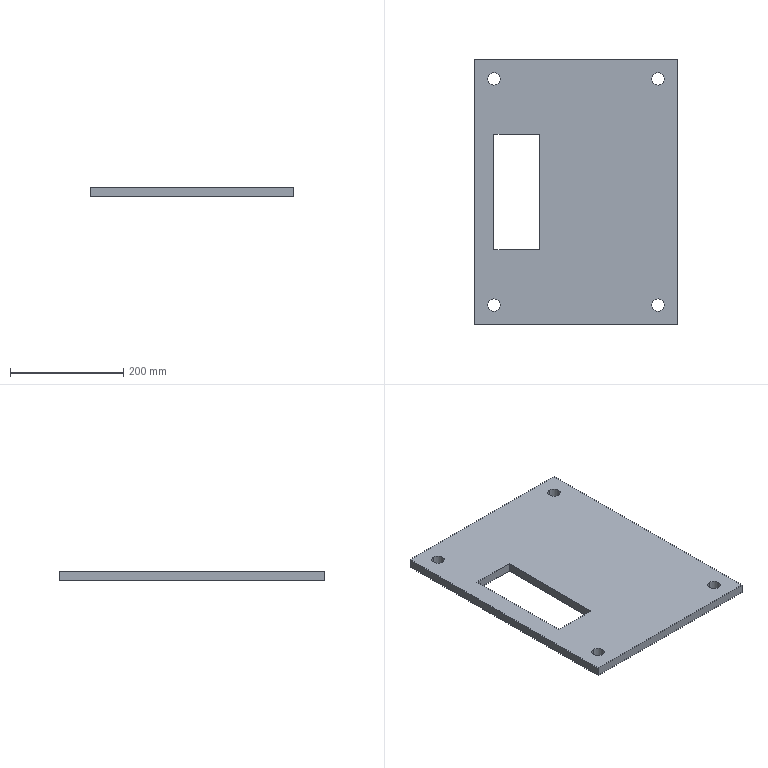Part | STEP file | 05-Base plate | 1 solid | 18 faces | box 360 x 470 x 16 mm | volume 2420472 mm3 | plane 10 | cylinder 8 | commonest cylinder face diameters 22 x8
STEP:
#1=CARTESIAN_POINT('',(0.,0.,0.));
#2=DIRECTION('',(0.,0.,1.));
#3=DIRECTION('',(1.,0.,0.));
#4=AXIS2_PLACEMENT_3D('',#1,#2,#3);
#5=CARTESIAN_POINT('',(35.,-446.,0.));
#6=VERTEX_POINT('',#5);
#7=CARTESIAN_POINT('',(35.,-446.,16.));
#8=VERTEX_POINT('',#7);
#9=CARTESIAN_POINT('',(35.,-446.,-44.));
#10=DIRECTION('',(0.,0.,1.));
#11=VECTOR('',#10,1.);
#12=LINE('',#9,#11);
#13=CARTESIAN_POINT('',(35.,-435.,-44.));
#14=DIRECTION('',(0.,0.,1.));
#15=DIRECTION('',(0.,-1.,0.));
#16=AXIS2_PLACEMENT_3D('',#13,#14,#15);
#17=CYLINDRICAL_SURFACE('',#16,11.);
#18=CARTESIAN_POINT('',(6.283,0.));
#19=DIRECTION('',(0.,1.));
#20=VECTOR('',#19,1.);
#21=LINE('',#18,#20);
#22=(GEOMETRIC_REPRESENTATION_CONTEXT(2)PARAMETRIC_REPRESENTATION_CONTEXT()REPRESENTATION_CONTEXT('',''));
#23=DEFINITIONAL_REPRESENTATION('',(#21),#22);
#24=PCURVE('',#17,#23);
#25=CARTESIAN_POINT('',(35.,-435.,-44.));
#26=DIRECTION('',(0.,0.,1.));
#27=DIRECTION('',(0.,-1.,0.));
#28=AXIS2_PLACEMENT_3D('',#25,#26,#27);
#29=CYLINDRICAL_SURFACE('',#28,11.);
#30=CARTESIAN_POINT('',(0.,0.));
#31=DIRECTION('',(0.,1.));
#32=VECTOR('',#31,1.);
#33=LINE('',#30,#32);
#34=(GEOMETRIC_REPRESENTATION_CONTEXT(2)PARAMETRIC_REPRESENTATION_CONTEXT()REPRESENTATION_CONTEXT('',''));
#35=DEFINITIONAL_REPRESENTATION('',(#33),#34);
#36=PCURVE('',#29,#35);
#37=SURFACE_CURVE('',#12,(#24,#36),.PCURVE_S1.);
#38=EDGE_CURVE('',#6,#8,#37,.T.);
#39=ORIENTED_EDGE('',*,*,#38,.T.);
#40=CARTESIAN_POINT('',(35.,-424.,16.));
#41=VERTEX_POINT('',#40);
#42=CARTESIAN_POINT('',(35.,-435.,16.));
#43=DIRECTION('',(0.,0.,1.));
#44=DIRECTION('',(0.,-1.,0.));
#45=AXIS2_PLACEMENT_3D('',#42,#43,#44);
#46=CIRCLE('',#45,11.);
#47=CARTESIAN_POINT('',(0.,60.));
#48=DIRECTION('',(1.,0.));
#49=VECTOR('',#48,1.);
#50=LINE('',#47,#49);
#51=(GEOMETRIC_REPRESENTATION_CONTEXT(2)PARAMETRIC_REPRESENTATION_CONTEXT()REPRESENTATION_CONTEXT('',''));
#52=DEFINITIONAL_REPRESENTATION('',(#50),#51);
#53=PCURVE('',#17,#52);
#54=CARTESIAN_POINT('',(0.,0.,16.));
#55=DIRECTION('',(0.,0.,1.));
#56=DIRECTION('',(1.,0.,0.));
#57=AXIS2_PLACEMENT_3D('',#54,#55,#56);
#58=PLANE('',#57);
#59=CARTESIAN_POINT('',(35.,-435.));
#60=DIRECTION('',(0.,-1.));
#61=AXIS2_PLACEMENT_2D('',#59,#60);
#62=CIRCLE('',#61,11.);
#63=(GEOMETRIC_REPRESENTATION_CONTEXT(2)PARAMETRIC_REPRESENTATION_CONTEXT()REPRESENTATION_CONTEXT('',''));
#64=DEFINITIONAL_REPRESENTATION('',(#62),#63);
#65=PCURVE('',#58,#64);
#66=SURFACE_CURVE('',#46,(#53,#65),.PCURVE_S1.);
#67=EDGE_CURVE('',#41,#8,#66,.T.);
#68=ORIENTED_EDGE('',*,*,#67,.F.);
#69=CARTESIAN_POINT('',(35.,-424.,0.));
#70=VERTEX_POINT('',#69);
#71=CARTESIAN_POINT('',(35.,-424.,-44.));
#72=DIRECTION('',(0.,0.,1.));
#73=VECTOR('',#72,1.);
#74=LINE('',#71,#73);
#75=CARTESIAN_POINT('',(3.142,0.));
#76=DIRECTION('',(0.,1.));
#77=VECTOR('',#76,1.);
#78=LINE('',#75,#77);
#79=(GEOMETRIC_REPRESENTATION_CONTEXT(2)PARAMETRIC_REPRESENTATION_CONTEXT()REPRESENTATION_CONTEXT('',''));
#80=DEFINITIONAL_REPRESENTATION('',(#78),#79);
#81=PCURVE('',#17,#80);
#82=CARTESIAN_POINT('',(3.142,0.));
#83=DIRECTION('',(0.,1.));
#84=VECTOR('',#83,1.);
#85=LINE('',#82,#84);
#86=(GEOMETRIC_REPRESENTATION_CONTEXT(2)PARAMETRIC_REPRESENTATION_CONTEXT()REPRESENTATION_CONTEXT('',''));
#87=DEFINITIONAL_REPRESENTATION('',(#85),#86);
#88=PCURVE('',#29,#87);
#89=SURFACE_CURVE('',#74,(#81,#88),.PCURVE_S1.);
#90=EDGE_CURVE('',#70,#41,#89,.T.);
#91=ORIENTED_EDGE('',*,*,#90,.F.);
#92=CARTESIAN_POINT('',(35.,-435.,0.));
#93=DIRECTION('',(0.,0.,1.));
#94=DIRECTION('',(0.,-1.,0.));
#95=AXIS2_PLACEMENT_3D('',#92,#93,#94);
#96=CIRCLE('',#95,11.);
#97=CARTESIAN_POINT('',(0.,44.));
#98=DIRECTION('',(1.,0.));
#99=VECTOR('',#98,1.);
#100=LINE('',#97,#99);
#101=(GEOMETRIC_REPRESENTATION_CONTEXT(2)PARAMETRIC_REPRESENTATION_CONTEXT()REPRESENTATION_CONTEXT('',''));
#102=DEFINITIONAL_REPRESENTATION('',(#100),#101);
#103=PCURVE('',#17,#102);
#104=CARTESIAN_POINT('',(0.,0.,0.));
#105=DIRECTION('',(0.,0.,1.));
#106=DIRECTION('',(1.,0.,0.));
#107=AXIS2_PLACEMENT_3D('',#104,#105,#106);
#108=PLANE('',#107);
#109=CARTESIAN_POINT('',(35.,-435.));
#110=DIRECTION('',(0.,-1.));
#111=AXIS2_PLACEMENT_2D('',#109,#110);
#112=CIRCLE('',#111,11.);
#113=(GEOMETRIC_REPRESENTATION_CONTEXT(2)PARAMETRIC_REPRESENTATION_CONTEXT()REPRESENTATION_CONTEXT('',''));
#114=DEFINITIONAL_REPRESENTATION('',(#112),#113);
#115=PCURVE('',#108,#114);
#116=SURFACE_CURVE('',#96,(#103,#115),.PCURVE_S1.);
#117=EDGE_CURVE('',#70,#6,#116,.T.);
#118=ORIENTED_EDGE('',*,*,#117,.T.);
#119=EDGE_LOOP('',(#39,#68,#91,#118));
#120=FACE_BOUND('',#119,.F.);
#121=ADVANCED_FACE('',(#120),#17,.F.);
#122=CARTESIAN_POINT('',(325.,-446.,0.));
#123=VERTEX_POINT('',#122);
#124=CARTESIAN_POINT('',(325.,-446.,16.));
#125=VERTEX_POINT('',#124);
#126=CARTESIAN_POINT('',(325.,-446.,-44.));
#127=DIRECTION('',(0.,0.,1.));
#128=VECTOR('',#127,1.);
#129=LINE('',#126,#128);
#130=CARTESIAN_POINT('',(325.,-435.,-44.));
#131=DIRECTION('',(0.,0.,1.));
#132=DIRECTION('',(0.,-1.,0.));
#133=AXIS2_PLACEMENT_3D('',#130,#131,#132);
#134=CYLINDRICAL_SURFACE('',#133,11.);
#135=CARTESIAN_POINT('',(6.283,0.));
#136=DIRECTION('',(0.,1.));
#137=VECTOR('',#136,1.);
#138=LINE('',#135,#137);
#139=(GEOMETRIC_REPRESENTATION_CONTEXT(2)PARAMETRIC_REPRESENTATION_CONTEXT()REPRESENTATION_CONTEXT('',''));
#140=DEFINITIONAL_REPRESENTATION('',(#138),#139);
#141=PCURVE('',#134,#140);
#142=CARTESIAN_POINT('',(325.,-435.,-44.));
#143=DIRECTION('',(0.,0.,1.));
#144=DIRECTION('',(0.,-1.,0.));
#145=AXIS2_PLACEMENT_3D('',#142,#143,#144);
#146=CYLINDRICAL_SURFACE('',#145,11.);
#147=CARTESIAN_POINT('',(0.,0.));
#148=DIRECTION('',(0.,1.));
#149=VECTOR('',#148,1.);
#150=LINE('',#147,#149);
#151=(GEOMETRIC_REPRESENTATION_CONTEXT(2)PARAMETRIC_REPRESENTATION_CONTEXT()REPRESENTATION_CONTEXT('',''));
#152=DEFINITIONAL_REPRESENTATION('',(#150),#151);
#153=PCURVE('',#146,#152);
#154=SURFACE_CURVE('',#129,(#141,#153),.PCURVE_S1.);
#155=EDGE_CURVE('',#123,#125,#154,.T.);
#156=ORIENTED_EDGE('',*,*,#155,.T.);
#157=CARTESIAN_POINT('',(325.,-424.,16.));
#158=VERTEX_POINT('',#157);
#159=CARTESIAN_POINT('',(325.,-435.,16.));
#160=DIRECTION('',(0.,0.,1.));
#161=DIRECTION('',(0.,-1.,0.));
#162=AXIS2_PLACEMENT_3D('',#159,#160,#161);
#163=CIRCLE('',#162,11.);
#164=CARTESIAN_POINT('',(0.,60.));
#165=DIRECTION('',(1.,0.));
#166=VECTOR('',#165,1.);
#167=LINE('',#164,#166);
#168=(GEOMETRIC_REPRESENTATION_CONTEXT(2)PARAMETRIC_REPRESENTATION_CONTEXT()REPRESENTATION_CONTEXT('',''));
#169=DEFINITIONAL_REPRESENTATION('',(#167),#168);
#170=PCURVE('',#134,#169);
#171=CARTESIAN_POINT('',(325.,-435.));
#172=DIRECTION('',(0.,-1.));
#173=AXIS2_PLACEMENT_2D('',#171,#172);
#174=CIRCLE('',#173,11.);
#175=(GEOMETRIC_REPRESENTATION_CONTEXT(2)PARAMETRIC_REPRESENTATION_CONTEXT()REPRESENTATION_CONTEXT('',''));
#176=DEFINITIONAL_REPRESENTATION('',(#174),#175);
#177=PCURVE('',#58,#176);
#178=SURFACE_CURVE('',#163,(#170,#177),.PCURVE_S1.);
#179=EDGE_CURVE('',#158,#125,#178,.T.);
#180=ORIENTED_EDGE('',*,*,#179,.F.);
#181=CARTESIAN_POINT('',(325.,-424.,0.));
#182=VERTEX_POINT('',#181);
#183=CARTESIAN_POINT('',(325.,-424.,-44.));
#184=DIRECTION('',(0.,0.,1.));
#185=VECTOR('',#184,1.);
#186=LINE('',#183,#185);
#187=CARTESIAN_POINT('',(3.142,0.));
#188=DIRECTION('',(0.,1.));
#189=VECTOR('',#188,1.);
#190=LINE('',#187,#189);
#191=(GEOMETRIC_REPRESENTATION_CONTEXT(2)PARAMETRIC_REPRESENTATION_CONTEXT()REPRESENTATION_CONTEXT('',''));
#192=DEFINITIONAL_REPRESENTATION('',(#190),#191);
#193=PCURVE('',#134,#192);
#194=CARTESIAN_POINT('',(3.142,0.));
#195=DIRECTION('',(0.,1.));
#196=VECTOR('',#195,1.);
#197=LINE('',#194,#196);
#198=(GEOMETRIC_REPRESENTATION_CONTEXT(2)PARAMETRIC_REPRESENTATION_CONTEXT()REPRESENTATION_CONTEXT('',''));
#199=DEFINITIONAL_REPRESENTATION('',(#197),#198);
#200=PCURVE('',#146,#199);
#201=SURFACE_CURVE('',#186,(#193,#200),.PCURVE_S1.);
#202=EDGE_CURVE('',#182,#158,#201,.T.);
#203=ORIENTED_EDGE('',*,*,#202,.F.);
#204=CARTESIAN_POINT('',(325.,-435.,0.));
#205=DIRECTION('',(0.,0.,1.));
#206=DIRECTION('',(0.,-1.,0.));
#207=AXIS2_PLACEMENT_3D('',#204,#205,#206);
#208=CIRCLE('',#207,11.);
#209=CARTESIAN_POINT('',(0.,44.));
#210=DIRECTION('',(1.,0.));
#211=VECTOR('',#210,1.);
#212=LINE('',#209,#211);
#213=(GEOMETRIC_REPRESENTATION_CONTEXT(2)PARAMETRIC_REPRESENTATION_CONTEXT()REPRESENTATION_CONTEXT('',''));
#214=DEFINITIONAL_REPRESENTATION('',(#212),#213);
#215=PCURVE('',#134,#214);
#216=CARTESIAN_POINT('',(325.,-435.));
#217=DIRECTION('',(0.,-1.));
#218=AXIS2_PLACEMENT_2D('',#216,#217);
#219=CIRCLE('',#218,11.);
#220=(GEOMETRIC_REPRESENTATION_CONTEXT(2)PARAMETRIC_REPRESENTATION_CONTEXT()REPRESENTATION_CONTEXT('',''));
#221=DEFINITIONAL_REPRESENTATION('',(#219),#220);
#222=PCURVE('',#108,#221);
#223=SURFACE_CURVE('',#208,(#215,#222),.PCURVE_S1.);
#224=EDGE_CURVE('',#182,#123,#223,.T.);
#225=ORIENTED_EDGE('',*,*,#224,.T.);
#226=EDGE_LOOP('',(#156,#180,#203,#225));
#227=FACE_BOUND('',#226,.F.);
#228=ADVANCED_FACE('',(#227),#134,.F.);
#229=CARTESIAN_POINT('',(325.,-46.,0.));
#230=VERTEX_POINT('',#229);
#231=CARTESIAN_POINT('',(325.,-46.,16.));
#232=VERTEX_POINT('',#231);
#233=CARTESIAN_POINT('',(325.,-46.,-44.));
#234=DIRECTION('',(0.,0.,1.));
#235=VECTOR('',#234,1.);
#236=LINE('',#233,#235);
#237=CARTESIAN_POINT('',(325.,-35.,-44.));
#238=DIRECTION('',(0.,0.,1.));
#239=DIRECTION('',(0.,-1.,0.));
#240=AXIS2_PLACEMENT_3D('',#237,#238,#239);
#241=CYLINDRICAL_SURFACE('',#240,11.);
#242=CARTESIAN_POINT('',(6.283,0.));
#243=DIRECTION('',(0.,1.));
#244=VECTOR('',#243,1.);
#245=LINE('',#242,#244);
#246=(GEOMETRIC_REPRESENTATION_CONTEXT(2)PARAMETRIC_REPRESENTATION_CONTEXT()REPRESENTATION_CONTEXT('',''));
#247=DEFINITIONAL_REPRESENTATION('',(#245),#246);
#248=PCURVE('',#241,#247);
#249=CARTESIAN_POINT('',(325.,-35.,-44.));
#250=DIRECTION('',(0.,0.,1.));
#251=DIRECTION('',(0.,-1.,0.));
#252=AXIS2_PLACEMENT_3D('',#249,#250,#251);
#253=CYLINDRICAL_SURFACE('',#252,11.);
#254=CARTESIAN_POINT('',(0.,0.));
#255=DIRECTION('',(0.,1.));
#256=VECTOR('',#255,1.);
#257=LINE('',#254,#256);
#258=(GEOMETRIC_REPRESENTATION_CONTEXT(2)PARAMETRIC_REPRESENTATION_CONTEXT()REPRESENTATION_CONTEXT('',''));
#259=DEFINITIONAL_REPRESENTATION('',(#257),#258);
#260=PCURVE('',#253,#259);
#261=SURFACE_CURVE('',#236,(#248,#260),.PCURVE_S1.);
#262=EDGE_CURVE('',#230,#232,#261,.T.);
#263=ORIENTED_EDGE('',*,*,#262,.T.);
#264=CARTESIAN_POINT('',(325.,-24.,16.));
#265=VERTEX_POINT('',#264);
#266=CARTESIAN_POINT('',(325.,-35.,16.));
#267=DIRECTION('',(0.,0.,1.));
#268=DIRECTION('',(0.,-1.,0.));
#269=AXIS2_PLACEMENT_3D('',#266,#267,#268);
#270=CIRCLE('',#269,11.);
#271=CARTESIAN_POINT('',(0.,60.));
#272=DIRECTION('',(1.,0.));
#273=VECTOR('',#272,1.);
#274=LINE('',#271,#273);
#275=(GEOMETRIC_REPRESENTATION_CONTEXT(2)PARAMETRIC_REPRESENTATION_CONTEXT()REPRESENTATION_CONTEXT('',''));
#276=DEFINITIONAL_REPRESENTATION('',(#274),#275);
#277=PCURVE('',#241,#276);
#278=CARTESIAN_POINT('',(325.,-35.));
#279=DIRECTION('',(0.,-1.));
#280=AXIS2_PLACEMENT_2D('',#278,#279);
#281=CIRCLE('',#280,11.);
#282=(GEOMETRIC_REPRESENTATION_CONTEXT(2)PARAMETRIC_REPRESENTATION_CONTEXT()REPRESENTATION_CONTEXT('',''));
#283=DEFINITIONAL_REPRESENTATION('',(#281),#282);
#284=PCURVE('',#58,#283);
#285=SURFACE_CURVE('',#270,(#277,#284),.PCURVE_S1.);
#286=EDGE_CURVE('',#265,#232,#285,.T.);
#287=ORIENTED_EDGE('',*,*,#286,.F.);
#288=CARTESIAN_POINT('',(325.,-24.,0.));
#289=VERTEX_POINT('',#288);
#290=CARTESIAN_POINT('',(325.,-24.,-44.));
#291=DIRECTION('',(0.,0.,1.));
#292=VECTOR('',#291,1.);
#293=LINE('',#290,#292);
#294=CARTESIAN_POINT('',(3.142,0.));
#295=DIRECTION('',(0.,1.));
#296=VECTOR('',#295,1.);
#297=LINE('',#294,#296);
#298=(GEOMETRIC_REPRESENTATION_CONTEXT(2)PARAMETRIC_REPRESENTATION_CONTEXT()REPRESENTATION_CONTEXT('',''));
#299=DEFINITIONAL_REPRESENTATION('',(#297),#298);
#300=PCURVE('',#241,#299);
#301=CARTESIAN_POINT('',(3.142,0.));
#302=DIRECTION('',(0.,1.));
#303=VECTOR('',#302,1.);
#304=LINE('',#301,#303);
#305=(GEOMETRIC_REPRESENTATION_CONTEXT(2)PARAMETRIC_REPRESENTATION_CONTEXT()REPRESENTATION_CONTEXT('',''));
#306=DEFINITIONAL_REPRESENTATION('',(#304),#305);
#307=PCURVE('',#253,#306);
#308=SURFACE_CURVE('',#293,(#300,#307),.PCURVE_S1.);
#309=EDGE_CURVE('',#289,#265,#308,.T.);
#310=ORIENTED_EDGE('',*,*,#309,.F.);
#311=CARTESIAN_POINT('',(325.,-35.,0.));
#312=DIRECTION('',(0.,0.,1.));
#313=DIRECTION('',(0.,-1.,0.));
#314=AXIS2_PLACEMENT_3D('',#311,#312,#313);
#315=CIRCLE('',#314,11.);
#316=CARTESIAN_POINT('',(0.,44.));
#317=DIRECTION('',(1.,0.));
#318=VECTOR('',#317,1.);
#319=LINE('',#316,#318);
#320=(GEOMETRIC_REPRESENTATION_CONTEXT(2)PARAMETRIC_REPRESENTATION_CONTEXT()REPRESENTATION_CONTEXT('',''));
#321=DEFINITIONAL_REPRESENTATION('',(#319),#320);
#322=PCURVE('',#241,#321);
#323=CARTESIAN_POINT('',(325.,-35.));
#324=DIRECTION('',(0.,-1.));
#325=AXIS2_PLACEMENT_2D('',#323,#324);
#326=CIRCLE('',#325,11.);
#327=(GEOMETRIC_REPRESENTATION_CONTEXT(2)PARAMETRIC_REPRESENTATION_CONTEXT()REPRESENTATION_CONTEXT('',''));
#328=DEFINITIONAL_REPRESENTATION('',(#326),#327);
#329=PCURVE('',#108,#328);
#330=SURFACE_CURVE('',#315,(#322,#329),.PCURVE_S1.);
#331=EDGE_CURVE('',#289,#230,#330,.T.);
#332=ORIENTED_EDGE('',*,*,#331,.T.);
#333=EDGE_LOOP('',(#263,#287,#310,#332));
#334=FACE_BOUND('',#333,.F.);
#335=ADVANCED_FACE('',(#334),#241,.F.);
#336=CARTESIAN_POINT('',(35.,-46.,0.));
#337=VERTEX_POINT('',#336);
#338=CARTESIAN_POINT('',(35.,-46.,16.));
#339=VERTEX_POINT('',#338);
#340=CARTESIAN_POINT('',(35.,-46.,-44.));
#341=DIRECTION('',(0.,0.,1.));
#342=VECTOR('',#341,1.);
#343=LINE('',#340,#342);
#344=CARTESIAN_POINT('',(35.,-35.,-44.));
#345=DIRECTION('',(0.,0.,1.));
#346=DIRECTION('',(0.,-1.,0.));
#347=AXIS2_PLACEMENT_3D('',#344,#345,#346);
#348=CYLINDRICAL_SURFACE('',#347,11.);
#349=CARTESIAN_POINT('',(6.283,0.));
#350=DIRECTION('',(0.,1.));
#351=VECTOR('',#350,1.);
#352=LINE('',#349,#351);
#353=(GEOMETRIC_REPRESENTATION_CONTEXT(2)PARAMETRIC_REPRESENTATION_CONTEXT()REPRESENTATION_CONTEXT('',''));
#354=DEFINITIONAL_REPRESENTATION('',(#352),#353);
#355=PCURVE('',#348,#354);
#356=CARTESIAN_POINT('',(35.,-35.,-44.));
#357=DIRECTION('',(0.,0.,1.));
#358=DIRECTION('',(0.,-1.,0.));
#359=AXIS2_PLACEMENT_3D('',#356,#357,#358);
#360=CYLINDRICAL_SURFACE('',#359,11.);
#361=CARTESIAN_POINT('',(0.,0.));
#362=DIRECTION('',(0.,1.));
#363=VECTOR('',#362,1.);
#364=LINE('',#361,#363);
#365=(GEOMETRIC_REPRESENTATION_CONTEXT(2)PARAMETRIC_REPRESENTATION_CONTEXT()REPRESENTATION_CONTEXT('',''));
#366=DEFINITIONAL_REPRESENTATION('',(#364),#365);
#367=PCURVE('',#360,#366);
#368=SURFACE_CURVE('',#343,(#355,#367),.PCURVE_S1.);
#369=EDGE_CURVE('',#337,#339,#368,.T.);
#370=ORIENTED_EDGE('',*,*,#369,.T.);
#371=CARTESIAN_POINT('',(35.,-24.,16.));
#372=VERTEX_POINT('',#371);
#373=CARTESIAN_POINT('',(35.,-35.,16.));
#374=DIRECTION('',(0.,0.,1.));
#375=DIRECTION('',(0.,-1.,0.));
#376=AXIS2_PLACEMENT_3D('',#373,#374,#375);
#377=CIRCLE('',#376,11.);
#378=CARTESIAN_POINT('',(0.,60.));
#379=DIRECTION('',(1.,0.));
#380=VECTOR('',#379,1.);
#381=LINE('',#378,#380);
#382=(GEOMETRIC_REPRESENTATION_CONTEXT(2)PARAMETRIC_REPRESENTATION_CONTEXT()REPRESENTATION_CONTEXT('',''));
#383=DEFINITIONAL_REPRESENTATION('',(#381),#382);
#384=PCURVE('',#348,#383);
#385=CARTESIAN_POINT('',(35.,-35.));
#386=DIRECTION('',(0.,-1.));
#387=AXIS2_PLACEMENT_2D('',#385,#386);
#388=CIRCLE('',#387,11.);
#389=(GEOMETRIC_REPRESENTATION_CONTEXT(2)PARAMETRIC_REPRESENTATION_CONTEXT()REPRESENTATION_CONTEXT('',''));
#390=DEFINITIONAL_REPRESENTATION('',(#388),#389);
#391=PCURVE('',#58,#390);
#392=SURFACE_CURVE('',#377,(#384,#391),.PCURVE_S1.);
#393=EDGE_CURVE('',#372,#339,#392,.T.);
#394=ORIENTED_EDGE('',*,*,#393,.F.);
#395=CARTESIAN_POINT('',(35.,-24.,0.));
#396=VERTEX_POINT('',#395);
#397=CARTESIAN_POINT('',(35.,-24.,-44.));
#398=DIRECTION('',(0.,0.,1.));
#399=VECTOR('',#398,1.);
#400=LINE('',#397,#399);
#401=CARTESIAN_POINT('',(3.142,0.));
#402=DIRECTION('',(0.,1.));
#403=VECTOR('',#402,1.);
#404=LINE('',#401,#403);
#405=(GEOMETRIC_REPRESENTATION_CONTEXT(2)PARAMETRIC_REPRESENTATION_CONTEXT()REPRESENTATION_CONTEXT('',''));
#406=DEFINITIONAL_REPRESENTATION('',(#404),#405);
#407=PCURVE('',#348,#406);
#408=CARTESIAN_POINT('',(3.142,0.));
#409=DIRECTION('',(0.,1.));
#410=VECTOR('',#409,1.);
#411=LINE('',#408,#410);
#412=(GEOMETRIC_REPRESENTATION_CONTEXT(2)PARAMETRIC_REPRESENTATION_CONTEXT()REPRESENTATION_CONTEXT('',''));
#413=DEFINITIONAL_REPRESENTATION('',(#411),#412);
#414=PCURVE('',#360,#413);
#415=SURFACE_CURVE('',#400,(#407,#414),.PCURVE_S1.);
#416=EDGE_CURVE('',#396,#372,#415,.T.);
#417=ORIENTED_EDGE('',*,*,#416,.F.);
#418=CARTESIAN_POINT('',(35.,-35.,0.));
#419=DIRECTION('',(0.,0.,1.));
#420=DIRECTION('',(0.,-1.,0.));
#421=AXIS2_PLACEMENT_3D('',#418,#419,#420);
#422=CIRCLE('',#421,11.);
#423=CARTESIAN_POINT('',(0.,44.));
#424=DIRECTION('',(1.,0.));
#425=VECTOR('',#424,1.);
#426=LINE('',#423,#425);
#427=(GEOMETRIC_REPRESENTATION_CONTEXT(2)PARAMETRIC_REPRESENTATION_CONTEXT()REPRESENTATION_CONTEXT('',''));
#428=DEFINITIONAL_REPRESENTATION('',(#426),#427);
#429=PCURVE('',#348,#428);
#430=CARTESIAN_POINT('',(35.,-35.));
#431=DIRECTION('',(0.,-1.));
#432=AXIS2_PLACEMENT_2D('',#430,#431);
#433=CIRCLE('',#432,11.);
#434=(GEOMETRIC_REPRESENTATION_CONTEXT(2)PARAMETRIC_REPRESENTATION_CONTEXT()REPRESENTATION_CONTEXT('',''));
#435=DEFINITIONAL_REPRESENTATION('',(#433),#434);
#436=PCURVE('',#108,#435);
#437=SURFACE_CURVE('',#422,(#429,#436),.PCURVE_S1.);
#438=EDGE_CURVE('',#396,#337,#437,.T.);
#439=ORIENTED_EDGE('',*,*,#438,.T.);
#440=EDGE_LOOP('',(#370,#394,#417,#439));
#441=FACE_BOUND('',#440,.F.);
#442=ADVANCED_FACE('',(#441),#348,.F.);
#443=CARTESIAN_POINT('',(0.,0.,0.));
#444=VERTEX_POINT('',#443);
#445=CARTESIAN_POINT('',(0.,-470.,0.));
#446=VERTEX_POINT('',#445);
#447=CARTESIAN_POINT('',(0.,0.,0.));
#448=DIRECTION('',(0.,-1.,0.));
#449=VECTOR('',#448,1.);
#450=LINE('',#447,#449);
#451=CARTESIAN_POINT('',(0.,0.,16.));
#452=DIRECTION('',(1.,0.,0.));
#453=DIRECTION('',(0.,1.,0.));
#454=AXIS2_PLACEMENT_3D('',#451,#452,#453);
#455=PLANE('',#454);
#456=CARTESIAN_POINT('',(0.,-16.));
#457=DIRECTION('',(-1.,0.));
#458=VECTOR('',#457,1.);
#459=LINE('',#456,#458);
#460=(GEOMETRIC_REPRESENTATION_CONTEXT(2)PARAMETRIC_REPRESENTATION_CONTEXT()REPRESENTATION_CONTEXT('',''));
#461=DEFINITIONAL_REPRESENTATION('',(#459),#460);
#462=PCURVE('',#455,#461);
#463=CARTESIAN_POINT('',(0.,0.));
#464=DIRECTION('',(0.,-1.));
#465=VECTOR('',#464,1.);
#466=LINE('',#463,#465);
#467=(GEOMETRIC_REPRESENTATION_CONTEXT(2)PARAMETRIC_REPRESENTATION_CONTEXT()REPRESENTATION_CONTEXT('',''));
#468=DEFINITIONAL_REPRESENTATION('',(#466),#467);
#469=PCURVE('',#108,#468);
#470=SURFACE_CURVE('',#450,(#462,#469),.PCURVE_S1.);
#471=EDGE_CURVE('',#444,#446,#470,.T.);
#472=ORIENTED_EDGE('',*,*,#471,.T.);
#473=CARTESIAN_POINT('',(0.,-470.,16.));
#474=VERTEX_POINT('',#473);
#475=CARTESIAN_POINT('',(0.,-470.,16.));
#476=DIRECTION('',(0.,0.,-1.));
#477=VECTOR('',#476,1.);
#478=LINE('',#475,#477);
#479=CARTESIAN_POINT('',(-470.,0.));
#480=DIRECTION('',(0.,-1.));
#481=VECTOR('',#480,1.);
#482=LINE('',#479,#481);
#483=(GEOMETRIC_REPRESENTATION_CONTEXT(2)PARAMETRIC_REPRESENTATION_CONTEXT()REPRESENTATION_CONTEXT('',''));
#484=DEFINITIONAL_REPRESENTATION('',(#482),#483);
#485=PCURVE('',#455,#484);
#486=CARTESIAN_POINT('',(0.,-470.,16.));
#487=DIRECTION('',(0.,1.,0.));
#488=DIRECTION('',(0.,0.,1.));
#489=AXIS2_PLACEMENT_3D('',#486,#487,#488);
#490=PLANE('',#489);
#491=CARTESIAN_POINT('',(0.,0.));
#492=DIRECTION('',(-1.,0.));
#493=VECTOR('',#492,1.);
#494=LINE('',#491,#493);
#495=(GEOMETRIC_REPRESENTATION_CONTEXT(2)PARAMETRIC_REPRESENTATION_CONTEXT()REPRESENTATION_CONTEXT('',''));
#496=DEFINITIONAL_REPRESENTATION('',(#494),#495);
#497=PCURVE('',#490,#496);
#498=SURFACE_CURVE('',#478,(#485,#497),.PCURVE_S1.);
#499=EDGE_CURVE('',#474,#446,#498,.T.);
#500=ORIENTED_EDGE('',*,*,#499,.F.);
#501=CARTESIAN_POINT('',(0.,0.,16.));
#502=VERTEX_POINT('',#501);
#503=CARTESIAN_POINT('',(0.,0.,16.));
#504=DIRECTION('',(0.,-1.,0.));
#505=VECTOR('',#504,1.);
#506=LINE('',#503,#505);
#507=CARTESIAN_POINT('',(0.,0.));
#508=DIRECTION('',(-1.,0.));
#509=VECTOR('',#508,1.);
#510=LINE('',#507,#509);
#511=(GEOMETRIC_REPRESENTATION_CONTEXT(2)PARAMETRIC_REPRESENTATION_CONTEXT()REPRESENTATION_CONTEXT('',''));
#512=DEFINITIONAL_REPRESENTATION('',(#510),#511);
#513=PCURVE('',#455,#512);
#514=CARTESIAN_POINT('',(0.,0.));
#515=DIRECTION('',(0.,-1.));
#516=VECTOR('',#515,1.);
#517=LINE('',#514,#516);
#518=(GEOMETRIC_REPRESENTATION_CONTEXT(2)PARAMETRIC_REPRESENTATION_CONTEXT()REPRESENTATION_CONTEXT('',''));
#519=DEFINITIONAL_REPRESENTATION('',(#517),#518);
#520=PCURVE('',#58,#519);
#521=SURFACE_CURVE('',#506,(#513,#520),.PCURVE_S1.);
#522=EDGE_CURVE('',#502,#474,#521,.T.);
#523=ORIENTED_EDGE('',*,*,#522,.F.);
#524=CARTESIAN_POINT('',(0.,0.,16.));
#525=DIRECTION('',(0.,0.,-1.));
#526=VECTOR('',#525,1.);
#527=LINE('',#524,#526);
#528=CARTESIAN_POINT('',(0.,0.));
#529=DIRECTION('',(0.,-1.));
#530=VECTOR('',#529,1.);
#531=LINE('',#528,#530);
#532=(GEOMETRIC_REPRESENTATION_CONTEXT(2)PARAMETRIC_REPRESENTATION_CONTEXT()REPRESENTATION_CONTEXT('',''));
#533=DEFINITIONAL_REPRESENTATION('',(#531),#532);
#534=PCURVE('',#455,#533);
#535=CARTESIAN_POINT('',(0.,0.,16.));
#536=DIRECTION('',(0.,-1.,0.));
#537=DIRECTION('',(0.,0.,-1.));
#538=AXIS2_PLACEMENT_3D('',#535,#536,#537);
#539=PLANE('',#538);
#540=CARTESIAN_POINT('',(0.,0.));
#541=DIRECTION('',(1.,0.));
#542=VECTOR('',#541,1.);
#543=LINE('',#540,#542);
#544=(GEOMETRIC_REPRESENTATION_CONTEXT(2)PARAMETRIC_REPRESENTATION_CONTEXT()REPRESENTATION_CONTEXT('',''));
#545=DEFINITIONAL_REPRESENTATION('',(#543),#544);
#546=PCURVE('',#539,#545);
#547=SURFACE_CURVE('',#527,(#534,#546),.PCURVE_S1.);
#548=EDGE_CURVE('',#502,#444,#547,.T.);
#549=ORIENTED_EDGE('',*,*,#548,.T.);
#550=EDGE_LOOP('',(#472,#500,#523,#549));
#551=FACE_BOUND('',#550,.T.);
#552=ADVANCED_FACE('',(#551),#455,.F.);
#553=CARTESIAN_POINT('',(360.,-470.,0.));
#554=VERTEX_POINT('',#553);
#555=CARTESIAN_POINT('',(0.,-470.,0.));
#556=DIRECTION('',(1.,0.,0.));
#557=VECTOR('',#556,1.);
#558=LINE('',#555,#557);
#559=CARTESIAN_POINT('',(-16.,0.));
#560=DIRECTION('',(0.,1.));
#561=VECTOR('',#560,1.);
#562=LINE('',#559,#561);
#563=(GEOMETRIC_REPRESENTATION_CONTEXT(2)PARAMETRIC_REPRESENTATION_CONTEXT()REPRESENTATION_CONTEXT('',''));
#564=DEFINITIONAL_REPRESENTATION('',(#562),#563);
#565=PCURVE('',#490,#564);
#566=CARTESIAN_POINT('',(0.,-470.));
#567=DIRECTION('',(1.,0.));
#568=VECTOR('',#567,1.);
#569=LINE('',#566,#568);
#570=(GEOMETRIC_REPRESENTATION_CONTEXT(2)PARAMETRIC_REPRESENTATION_CONTEXT()REPRESENTATION_CONTEXT('',''));
#571=DEFINITIONAL_REPRESENTATION('',(#569),#570);
#572=PCURVE('',#108,#571);
#573=SURFACE_CURVE('',#558,(#565,#572),.PCURVE_S1.);
#574=EDGE_CURVE('',#446,#554,#573,.T.);
#575=ORIENTED_EDGE('',*,*,#574,.T.);
#576=CARTESIAN_POINT('',(360.,-470.,16.));
#577=VERTEX_POINT('',#576);
#578=CARTESIAN_POINT('',(360.,-470.,16.));
#579=DIRECTION('',(0.,0.,-1.));
#580=VECTOR('',#579,1.);
#581=LINE('',#578,#580);
#582=CARTESIAN_POINT('',(0.,360.));
#583=DIRECTION('',(-1.,0.));
#584=VECTOR('',#583,1.);
#585=LINE('',#582,#584);
#586=(GEOMETRIC_REPRESENTATION_CONTEXT(2)PARAMETRIC_REPRESENTATION_CONTEXT()REPRESENTATION_CONTEXT('',''));
#587=DEFINITIONAL_REPRESENTATION('',(#585),#586);
#588=PCURVE('',#490,#587);
#589=CARTESIAN_POINT('',(360.,0.,16.));
#590=DIRECTION('',(-1.,0.,0.));
#591=DIRECTION('',(0.,-1.,0.));
#592=AXIS2_PLACEMENT_3D('',#589,#590,#591);
#593=PLANE('',#592);
#594=CARTESIAN_POINT('',(470.,0.));
#595=DIRECTION('',(0.,-1.));
#596=VECTOR('',#595,1.);
#597=LINE('',#594,#596);
#598=(GEOMETRIC_REPRESENTATION_CONTEXT(2)PARAMETRIC_REPRESENTATION_CONTEXT()REPRESENTATION_CONTEXT('',''));
#599=DEFINITIONAL_REPRESENTATION('',(#597),#598);
#600=PCURVE('',#593,#599);
#601=SURFACE_CURVE('',#581,(#588,#600),.PCURVE_S1.);
#602=EDGE_CURVE('',#577,#554,#601,.T.);
#603=ORIENTED_EDGE('',*,*,#602,.F.);
#604=CARTESIAN_POINT('',(0.,-470.,16.));
#605=DIRECTION('',(1.,0.,0.));
#606=VECTOR('',#605,1.);
#607=LINE('',#604,#606);
#608=CARTESIAN_POINT('',(0.,0.));
#609=DIRECTION('',(0.,1.));
#610=VECTOR('',#609,1.);
#611=LINE('',#608,#610);
#612=(GEOMETRIC_REPRESENTATION_CONTEXT(2)PARAMETRIC_REPRESENTATION_CONTEXT()REPRESENTATION_CONTEXT('',''));
#613=DEFINITIONAL_REPRESENTATION('',(#611),#612);
#614=PCURVE('',#490,#613);
#615=CARTESIAN_POINT('',(0.,-470.));
#616=DIRECTION('',(1.,0.));
#617=VECTOR('',#616,1.);
#618=LINE('',#615,#617);
#619=(GEOMETRIC_REPRESENTATION_CONTEXT(2)PARAMETRIC_REPRESENTATION_CONTEXT()REPRESENTATION_CONTEXT('',''));
#620=DEFINITIONAL_REPRESENTATION('',(#618),#619);
#621=PCURVE('',#58,#620);
#622=SURFACE_CURVE('',#607,(#614,#621),.PCURVE_S1.);
#623=EDGE_CURVE('',#474,#577,#622,.T.);
#624=ORIENTED_EDGE('',*,*,#623,.F.);
#625=ORIENTED_EDGE('',*,*,#499,.T.);
#626=EDGE_LOOP('',(#575,#603,#624,#625));
#627=FACE_BOUND('',#626,.T.);
#628=ADVANCED_FACE('',(#627),#490,.F.);
#629=CARTESIAN_POINT('',(360.,0.,0.));
#630=VERTEX_POINT('',#629);
#631=CARTESIAN_POINT('',(360.,0.,0.));
#632=DIRECTION('',(0.,1.,0.));
#633=VECTOR('',#632,1.);
#634=LINE('',#631,#633);
#635=CARTESIAN_POINT('',(0.,-16.));
#636=DIRECTION('',(-1.,0.));
#637=VECTOR('',#636,1.);
#638=LINE('',#635,#637);
#639=(GEOMETRIC_REPRESENTATION_CONTEXT(2)PARAMETRIC_REPRESENTATION_CONTEXT()REPRESENTATION_CONTEXT('',''));
#640=DEFINITIONAL_REPRESENTATION('',(#638),#639);
#641=PCURVE('',#593,#640);
#642=CARTESIAN_POINT('',(360.,0.));
#643=DIRECTION('',(0.,1.));
#644=VECTOR('',#643,1.);
#645=LINE('',#642,#644);
#646=(GEOMETRIC_REPRESENTATION_CONTEXT(2)PARAMETRIC_REPRESENTATION_CONTEXT()REPRESENTATION_CONTEXT('',''));
#647=DEFINITIONAL_REPRESENTATION('',(#645),#646);
#648=PCURVE('',#108,#647);
#649=SURFACE_CURVE('',#634,(#641,#648),.PCURVE_S1.);
#650=EDGE_CURVE('',#554,#630,#649,.T.);
#651=ORIENTED_EDGE('',*,*,#650,.T.);
#652=CARTESIAN_POINT('',(360.,0.,16.));
#653=VERTEX_POINT('',#652);
#654=CARTESIAN_POINT('',(360.,0.,16.));
#655=DIRECTION('',(0.,0.,-1.));
#656=VECTOR('',#655,1.);
#657=LINE('',#654,#656);
#658=CARTESIAN_POINT('',(0.,0.));
#659=DIRECTION('',(0.,-1.));
#660=VECTOR('',#659,1.);
#661=LINE('',#658,#660);
#662=(GEOMETRIC_REPRESENTATION_CONTEXT(2)PARAMETRIC_REPRESENTATION_CONTEXT()REPRESENTATION_CONTEXT('',''));
#663=DEFINITIONAL_REPRESENTATION('',(#661),#662);
#664=PCURVE('',#593,#663);
#665=CARTESIAN_POINT('',(0.,360.));
#666=DIRECTION('',(1.,0.));
#667=VECTOR('',#666,1.);
#668=LINE('',#665,#667);
#669=(GEOMETRIC_REPRESENTATION_CONTEXT(2)PARAMETRIC_REPRESENTATION_CONTEXT()REPRESENTATION_CONTEXT('',''));
#670=DEFINITIONAL_REPRESENTATION('',(#668),#669);
#671=PCURVE('',#539,#670);
#672=SURFACE_CURVE('',#657,(#664,#671),.PCURVE_S1.);
#673=EDGE_CURVE('',#653,#630,#672,.T.);
#674=ORIENTED_EDGE('',*,*,#673,.F.);
#675=CARTESIAN_POINT('',(360.,0.,16.));
#676=DIRECTION('',(0.,1.,0.));
#677=VECTOR('',#676,1.);
#678=LINE('',#675,#677);
#679=CARTESIAN_POINT('',(0.,0.));
#680=DIRECTION('',(-1.,0.));
#681=VECTOR('',#680,1.);
#682=LINE('',#679,#681);
#683=(GEOMETRIC_REPRESENTATION_CONTEXT(2)PARAMETRIC_REPRESENTATION_CONTEXT()REPRESENTATION_CONTEXT('',''));
#684=DEFINITIONAL_REPRESENTATION('',(#682),#683);
#685=PCURVE('',#593,#684);
#686=CARTESIAN_POINT('',(360.,0.));
#687=DIRECTION('',(0.,1.));
#688=VECTOR('',#687,1.);
#689=LINE('',#686,#688);
#690=(GEOMETRIC_REPRESENTATION_CONTEXT(2)PARAMETRIC_REPRESENTATION_CONTEXT()REPRESENTATION_CONTEXT('',''));
#691=DEFINITIONAL_REPRESENTATION('',(#689),#690);
#692=PCURVE('',#58,#691);
#693=SURFACE_CURVE('',#678,(#685,#692),.PCURVE_S1.);
#694=EDGE_CURVE('',#577,#653,#693,.T.);
#695=ORIENTED_EDGE('',*,*,#694,.F.);
#696=ORIENTED_EDGE('',*,*,#602,.T.);
#697=EDGE_LOOP('',(#651,#674,#695,#696));
#698=FACE_BOUND('',#697,.T.);
#699=ADVANCED_FACE('',(#698),#593,.F.);
#700=CARTESIAN_POINT('',(0.,0.,0.));
#701=DIRECTION('',(-1.,0.,0.));
#702=VECTOR('',#701,1.);
#703=LINE('',#700,#702);
#704=CARTESIAN_POINT('',(16.,0.));
#705=DIRECTION('',(0.,-1.));
#706=VECTOR('',#705,1.);
#707=LINE('',#704,#706);
#708=(GEOMETRIC_REPRESENTATION_CONTEXT(2)PARAMETRIC_REPRESENTATION_CONTEXT()REPRESENTATION_CONTEXT('',''));
#709=DEFINITIONAL_REPRESENTATION('',(#707),#708);
#710=PCURVE('',#539,#709);
#711=CARTESIAN_POINT('',(0.,0.));
#712=DIRECTION('',(-1.,0.));
#713=VECTOR('',#712,1.);
#714=LINE('',#711,#713);
#715=(GEOMETRIC_REPRESENTATION_CONTEXT(2)PARAMETRIC_REPRESENTATION_CONTEXT()REPRESENTATION_CONTEXT('',''));
#716=DEFINITIONAL_REPRESENTATION('',(#714),#715);
#717=PCURVE('',#108,#716);
#718=SURFACE_CURVE('',#703,(#710,#717),.PCURVE_S1.);
#719=EDGE_CURVE('',#630,#444,#718,.T.);
#720=ORIENTED_EDGE('',*,*,#719,.T.);
#721=ORIENTED_EDGE('',*,*,#548,.F.);
#722=CARTESIAN_POINT('',(0.,0.,16.));
#723=DIRECTION('',(-1.,0.,0.));
#724=VECTOR('',#723,1.);
#725=LINE('',#722,#724);
#726=CARTESIAN_POINT('',(0.,0.));
#727=DIRECTION('',(0.,-1.));
#728=VECTOR('',#727,1.);
#729=LINE('',#726,#728);
#730=(GEOMETRIC_REPRESENTATION_CONTEXT(2)PARAMETRIC_REPRESENTATION_CONTEXT()REPRESENTATION_CONTEXT('',''));
#731=DEFINITIONAL_REPRESENTATION('',(#729),#730);
#732=PCURVE('',#539,#731);
#733=CARTESIAN_POINT('',(0.,0.));
#734=DIRECTION('',(-1.,0.));
#735=VECTOR('',#734,1.);
#736=LINE('',#733,#735);
#737=(GEOMETRIC_REPRESENTATION_CONTEXT(2)PARAMETRIC_REPRESENTATION_CONTEXT()REPRESENTATION_CONTEXT('',''));
#738=DEFINITIONAL_REPRESENTATION('',(#736),#737);
#739=PCURVE('',#58,#738);
#740=SURFACE_CURVE('',#725,(#732,#739),.PCURVE_S1.);
#741=EDGE_CURVE('',#653,#502,#740,.T.);
#742=ORIENTED_EDGE('',*,*,#741,.F.);
#743=ORIENTED_EDGE('',*,*,#673,.T.);
#744=EDGE_LOOP('',(#720,#721,#742,#743));
#745=FACE_BOUND('',#744,.T.);
#746=ADVANCED_FACE('',(#745),#539,.F.);
#747=CARTESIAN_POINT('',(35.,-132.5,16.));
#748=VERTEX_POINT('',#747);
#749=CARTESIAN_POINT('',(35.,-337.5,16.));
#750=VERTEX_POINT('',#749);
#751=CARTESIAN_POINT('',(35.,-132.5,16.));
#752=DIRECTION('',(0.,-1.,0.));
#753=VECTOR('',#752,1.);
#754=LINE('',#751,#753);
#755=CARTESIAN_POINT('',(35.,-132.5));
#756=DIRECTION('',(0.,-1.));
#757=VECTOR('',#756,1.);
#758=LINE('',#755,#757);
#759=(GEOMETRIC_REPRESENTATION_CONTEXT(2)PARAMETRIC_REPRESENTATION_CONTEXT()REPRESENTATION_CONTEXT('',''));
#760=DEFINITIONAL_REPRESENTATION('',(#758),#759);
#761=PCURVE('',#58,#760);
#762=CARTESIAN_POINT('',(35.,-132.5,-44.));
#763=DIRECTION('',(-1.,0.,0.));
#764=DIRECTION('',(0.,1.,0.));
#765=AXIS2_PLACEMENT_3D('',#762,#763,#764);
#766=PLANE('',#765);
#767=CARTESIAN_POINT('',(0.,-60.));
#768=DIRECTION('',(-1.,0.));
#769=VECTOR('',#768,1.);
#770=LINE('',#767,#769);
#771=(GEOMETRIC_REPRESENTATION_CONTEXT(2)PARAMETRIC_REPRESENTATION_CONTEXT()REPRESENTATION_CONTEXT('',''));
#772=DEFINITIONAL_REPRESENTATION('',(#770),#771);
#773=PCURVE('',#766,#772);
#774=SURFACE_CURVE('',#754,(#761,#773),.PCURVE_S1.);
#775=EDGE_CURVE('',#748,#750,#774,.T.);
#776=ORIENTED_EDGE('',*,*,#775,.F.);
#777=CARTESIAN_POINT('',(115.,-132.5,16.));
#778=VERTEX_POINT('',#777);
#779=CARTESIAN_POINT('',(35.,-132.5,16.));
#780=DIRECTION('',(-1.,0.,0.));
#781=VECTOR('',#780,1.);
#782=LINE('',#779,#781);
#783=CARTESIAN_POINT('',(35.,-132.5));
#784=DIRECTION('',(-1.,0.));
#785=VECTOR('',#784,1.);
#786=LINE('',#783,#785);
#787=(GEOMETRIC_REPRESENTATION_CONTEXT(2)PARAMETRIC_REPRESENTATION_CONTEXT()REPRESENTATION_CONTEXT('',''));
#788=DEFINITIONAL_REPRESENTATION('',(#786),#787);
#789=PCURVE('',#58,#788);
#790=CARTESIAN_POINT('',(35.,-132.5,-44.));
#791=DIRECTION('',(0.,1.,0.));
#792=DIRECTION('',(1.,0.,0.));
#793=AXIS2_PLACEMENT_3D('',#790,#791,#792);
#794=PLANE('',#793);
#795=CARTESIAN_POINT('',(0.,-60.));
#796=DIRECTION('',(-1.,0.));
#797=VECTOR('',#796,1.);
#798=LINE('',#795,#797);
#799=(GEOMETRIC_REPRESENTATION_CONTEXT(2)PARAMETRIC_REPRESENTATION_CONTEXT()REPRESENTATION_CONTEXT('',''));
#800=DEFINITIONAL_REPRESENTATION('',(#798),#799);
#801=PCURVE('',#794,#800);
#802=SURFACE_CURVE('',#782,(#789,#801),.PCURVE_S1.);
#803=EDGE_CURVE('',#778,#748,#802,.T.);
#804=ORIENTED_EDGE('',*,*,#803,.F.);
#805=CARTESIAN_POINT('',(115.,-337.5,16.));
#806=VERTEX_POINT('',#805);
#807=CARTESIAN_POINT('',(115.,-132.5,16.));
#808=DIRECTION('',(0.,1.,0.));
#809=VECTOR('',#808,1.);
#810=LINE('',#807,#809);
#811=CARTESIAN_POINT('',(115.,-132.5));
#812=DIRECTION('',(0.,1.));
#813=VECTOR('',#812,1.);
#814=LINE('',#811,#813);
#815=(GEOMETRIC_REPRESENTATION_CONTEXT(2)PARAMETRIC_REPRESENTATION_CONTEXT()REPRESENTATION_CONTEXT('',''));
#816=DEFINITIONAL_REPRESENTATION('',(#814),#815);
#817=PCURVE('',#58,#816);
#818=CARTESIAN_POINT('',(115.,-132.5,-44.));
#819=DIRECTION('',(1.,0.,0.));
#820=DIRECTION('',(0.,-1.,0.));
#821=AXIS2_PLACEMENT_3D('',#818,#819,#820);
#822=PLANE('',#821);
#823=CARTESIAN_POINT('',(0.,-60.));
#824=DIRECTION('',(-1.,0.));
#825=VECTOR('',#824,1.);
#826=LINE('',#823,#825);
#827=(GEOMETRIC_REPRESENTATION_CONTEXT(2)PARAMETRIC_REPRESENTATION_CONTEXT()REPRESENTATION_CONTEXT('',''));
#828=DEFINITIONAL_REPRESENTATION('',(#826),#827);
#829=PCURVE('',#822,#828);
#830=SURFACE_CURVE('',#810,(#817,#829),.PCURVE_S1.);
#831=EDGE_CURVE('',#806,#778,#830,.T.);
#832=ORIENTED_EDGE('',*,*,#831,.F.);
#833=CARTESIAN_POINT('',(35.,-337.5,16.));
#834=DIRECTION('',(1.,0.,0.));
#835=VECTOR('',#834,1.);
#836=LINE('',#833,#835);
#837=CARTESIAN_POINT('',(35.,-337.5));
#838=DIRECTION('',(1.,0.));
#839=VECTOR('',#838,1.);
#840=LINE('',#837,#839);
#841=(GEOMETRIC_REPRESENTATION_CONTEXT(2)PARAMETRIC_REPRESENTATION_CONTEXT()REPRESENTATION_CONTEXT('',''));
#842=DEFINITIONAL_REPRESENTATION('',(#840),#841);
#843=PCURVE('',#58,#842);
#844=CARTESIAN_POINT('',(35.,-337.5,-44.));
#845=DIRECTION('',(0.,-1.,0.));
#846=DIRECTION('',(-1.,0.,0.));
#847=AXIS2_PLACEMENT_3D('',#844,#845,#846);
#848=PLANE('',#847);
#849=CARTESIAN_POINT('',(0.,-60.));
#850=DIRECTION('',(-1.,0.));
#851=VECTOR('',#850,1.);
#852=LINE('',#849,#851);
#853=(GEOMETRIC_REPRESENTATION_CONTEXT(2)PARAMETRIC_REPRESENTATION_CONTEXT()REPRESENTATION_CONTEXT('',''));
#854=DEFINITIONAL_REPRESENTATION('',(#852),#853);
#855=PCURVE('',#848,#854);
#856=SURFACE_CURVE('',#836,(#843,#855),.PCURVE_S1.);
#857=EDGE_CURVE('',#750,#806,#856,.T.);
#858=ORIENTED_EDGE('',*,*,#857,.F.);
#859=EDGE_LOOP('',(#776,#804,#832,#858));
#860=FACE_BOUND('',#859,.T.);
#861=CARTESIAN_POINT('',(35.,-435.,16.));
#862=DIRECTION('',(0.,0.,1.));
#863=DIRECTION('',(0.,-1.,0.));
#864=AXIS2_PLACEMENT_3D('',#861,#862,#863);
#865=CIRCLE('',#864,11.);
#866=CARTESIAN_POINT('',(35.,-435.));
#867=DIRECTION('',(0.,-1.));
#868=AXIS2_PLACEMENT_2D('',#866,#867);
#869=CIRCLE('',#868,11.);
#870=(GEOMETRIC_REPRESENTATION_CONTEXT(2)PARAMETRIC_REPRESENTATION_CONTEXT()REPRESENTATION_CONTEXT('',''));
#871=DEFINITIONAL_REPRESENTATION('',(#869),#870);
#872=PCURVE('',#58,#871);
#873=CARTESIAN_POINT('',(0.,60.));
#874=DIRECTION('',(1.,0.));
#875=VECTOR('',#874,1.);
#876=LINE('',#873,#875);
#877=(GEOMETRIC_REPRESENTATION_CONTEXT(2)PARAMETRIC_REPRESENTATION_CONTEXT()REPRESENTATION_CONTEXT('',''));
#878=DEFINITIONAL_REPRESENTATION('',(#876),#877);
#879=PCURVE('',#29,#878);
#880=SURFACE_CURVE('',#865,(#872,#879),.PCURVE_S1.);
#881=EDGE_CURVE('',#8,#41,#880,.T.);
#882=ORIENTED_EDGE('',*,*,#881,.F.);
#883=ORIENTED_EDGE('',*,*,#67,.F.);
#884=EDGE_LOOP('',(#882,#883));
#885=FACE_BOUND('',#884,.T.);
#886=CARTESIAN_POINT('',(325.,-435.,16.));
#887=DIRECTION('',(0.,0.,1.));
#888=DIRECTION('',(0.,-1.,0.));
#889=AXIS2_PLACEMENT_3D('',#886,#887,#888);
#890=CIRCLE('',#889,11.);
#891=CARTESIAN_POINT('',(325.,-435.));
#892=DIRECTION('',(0.,-1.));
#893=AXIS2_PLACEMENT_2D('',#891,#892);
#894=CIRCLE('',#893,11.);
#895=(GEOMETRIC_REPRESENTATION_CONTEXT(2)PARAMETRIC_REPRESENTATION_CONTEXT()REPRESENTATION_CONTEXT('',''));
#896=DEFINITIONAL_REPRESENTATION('',(#894),#895);
#897=PCURVE('',#58,#896);
#898=CARTESIAN_POINT('',(0.,60.));
#899=DIRECTION('',(1.,0.));
#900=VECTOR('',#899,1.);
#901=LINE('',#898,#900);
#902=(GEOMETRIC_REPRESENTATION_CONTEXT(2)PARAMETRIC_REPRESENTATION_CONTEXT()REPRESENTATION_CONTEXT('',''));
#903=DEFINITIONAL_REPRESENTATION('',(#901),#902);
#904=PCURVE('',#146,#903);
#905=SURFACE_CURVE('',#890,(#897,#904),.PCURVE_S1.);
#906=EDGE_CURVE('',#125,#158,#905,.T.);
#907=ORIENTED_EDGE('',*,*,#906,.F.);
#908=ORIENTED_EDGE('',*,*,#179,.F.);
#909=EDGE_LOOP('',(#907,#908));
#910=FACE_BOUND('',#909,.T.);
#911=CARTESIAN_POINT('',(325.,-35.,16.));
#912=DIRECTION('',(0.,0.,1.));
#913=DIRECTION('',(0.,-1.,0.));
#914=AXIS2_PLACEMENT_3D('',#911,#912,#913);
#915=CIRCLE('',#914,11.);
#916=CARTESIAN_POINT('',(325.,-35.));
#917=DIRECTION('',(0.,-1.));
#918=AXIS2_PLACEMENT_2D('',#916,#917);
#919=CIRCLE('',#918,11.);
#920=(GEOMETRIC_REPRESENTATION_CONTEXT(2)PARAMETRIC_REPRESENTATION_CONTEXT()REPRESENTATION_CONTEXT('',''));
#921=DEFINITIONAL_REPRESENTATION('',(#919),#920);
#922=PCURVE('',#58,#921);
#923=CARTESIAN_POINT('',(0.,60.));
#924=DIRECTION('',(1.,0.));
#925=VECTOR('',#924,1.);
#926=LINE('',#923,#925);
#927=(GEOMETRIC_REPRESENTATION_CONTEXT(2)PARAMETRIC_REPRESENTATION_CONTEXT()REPRESENTATION_CONTEXT('',''));
#928=DEFINITIONAL_REPRESENTATION('',(#926),#927);
#929=PCURVE('',#253,#928);
#930=SURFACE_CURVE('',#915,(#922,#929),.PCURVE_S1.);
#931=EDGE_CURVE('',#232,#265,#930,.T.);
#932=ORIENTED_EDGE('',*,*,#931,.F.);
#933=ORIENTED_EDGE('',*,*,#286,.F.);
#934=EDGE_LOOP('',(#932,#933));
#935=FACE_BOUND('',#934,.T.);
#936=CARTESIAN_POINT('',(35.,-35.,16.));
#937=DIRECTION('',(0.,0.,1.));
#938=DIRECTION('',(0.,-1.,0.));
#939=AXIS2_PLACEMENT_3D('',#936,#937,#938);
#940=CIRCLE('',#939,11.);
#941=CARTESIAN_POINT('',(35.,-35.));
#942=DIRECTION('',(0.,-1.));
#943=AXIS2_PLACEMENT_2D('',#941,#942);
#944=CIRCLE('',#943,11.);
#945=(GEOMETRIC_REPRESENTATION_CONTEXT(2)PARAMETRIC_REPRESENTATION_CONTEXT()REPRESENTATION_CONTEXT('',''));
#946=DEFINITIONAL_REPRESENTATION('',(#944),#945);
#947=PCURVE('',#58,#946);
#948=CARTESIAN_POINT('',(0.,60.));
#949=DIRECTION('',(1.,0.));
#950=VECTOR('',#949,1.);
#951=LINE('',#948,#950);
#952=(GEOMETRIC_REPRESENTATION_CONTEXT(2)PARAMETRIC_REPRESENTATION_CONTEXT()REPRESENTATION_CONTEXT('',''));
#953=DEFINITIONAL_REPRESENTATION('',(#951),#952);
#954=PCURVE('',#360,#953);
#955=SURFACE_CURVE('',#940,(#947,#954),.PCURVE_S1.);
#956=EDGE_CURVE('',#339,#372,#955,.T.);
#957=ORIENTED_EDGE('',*,*,#956,.F.);
#958=ORIENTED_EDGE('',*,*,#393,.F.);
#959=EDGE_LOOP('',(#957,#958));
#960=FACE_BOUND('',#959,.T.);
#961=ORIENTED_EDGE('',*,*,#522,.T.);
#962=ORIENTED_EDGE('',*,*,#623,.T.);
#963=ORIENTED_EDGE('',*,*,#694,.T.);
#964=ORIENTED_EDGE('',*,*,#741,.T.);
#965=EDGE_LOOP('',(#961,#962,#963,#964));
#966=FACE_BOUND('',#965,.T.);
#967=ADVANCED_FACE('',(#860,#885,#910,#935,#960,#966),#58,.T.);
#968=CARTESIAN_POINT('',(115.,-132.5,0.));
#969=VERTEX_POINT('',#968);
#970=CARTESIAN_POINT('',(35.,-132.5,0.));
#971=VERTEX_POINT('',#970);
#972=CARTESIAN_POINT('',(0.,-132.5,0.));
#973=DIRECTION('',(-1.,0.,0.));
#974=VECTOR('',#973,1.);
#975=LINE('',#972,#974);
#976=CARTESIAN_POINT('',(0.,-132.5));
#977=DIRECTION('',(-1.,0.));
#978=VECTOR('',#977,1.);
#979=LINE('',#976,#978);
#980=(GEOMETRIC_REPRESENTATION_CONTEXT(2)PARAMETRIC_REPRESENTATION_CONTEXT()REPRESENTATION_CONTEXT('',''));
#981=DEFINITIONAL_REPRESENTATION('',(#979),#980);
#982=PCURVE('',#108,#981);
#983=CARTESIAN_POINT('',(-35.,-44.));
#984=DIRECTION('',(-1.,0.));
#985=VECTOR('',#984,1.);
#986=LINE('',#983,#985);
#987=(GEOMETRIC_REPRESENTATION_CONTEXT(2)PARAMETRIC_REPRESENTATION_CONTEXT()REPRESENTATION_CONTEXT('',''));
#988=DEFINITIONAL_REPRESENTATION('',(#986),#987);
#989=PCURVE('',#794,#988);
#990=SURFACE_CURVE('',#975,(#982,#989),.PCURVE_S1.);
#991=EDGE_CURVE('',#969,#971,#990,.T.);
#992=ORIENTED_EDGE('',*,*,#991,.T.);
#993=CARTESIAN_POINT('',(35.,-337.5,0.));
#994=VERTEX_POINT('',#993);
#995=CARTESIAN_POINT('',(35.,0.,0.));
#996=DIRECTION('',(0.,-1.,0.));
#997=VECTOR('',#996,1.);
#998=LINE('',#995,#997);
#999=CARTESIAN_POINT('',(35.,0.));
#1000=DIRECTION('',(0.,-1.));
#1001=VECTOR('',#1000,1.);
#1002=LINE('',#999,#1001);
#1003=(GEOMETRIC_REPRESENTATION_CONTEXT(2)PARAMETRIC_REPRESENTATION_CONTEXT()REPRESENTATION_CONTEXT('',''));
#1004=DEFINITIONAL_REPRESENTATION('',(#1002),#1003);
#1005=PCURVE('',#108,#1004);
#1006=CARTESIAN_POINT('',(132.5,-44.));
#1007=DIRECTION('',(-1.,0.));
#1008=VECTOR('',#1007,1.);
#1009=LINE('',#1006,#1008);
#1010=(GEOMETRIC_REPRESENTATION_CONTEXT(2)PARAMETRIC_REPRESENTATION_CONTEXT()REPRESENTATION_CONTEXT('',''));
#1011=DEFINITIONAL_REPRESENTATION('',(#1009),#1010);
#1012=PCURVE('',#766,#1011);
#1013=SURFACE_CURVE('',#998,(#1005,#1012),.PCURVE_S1.);
#1014=EDGE_CURVE('',#971,#994,#1013,.T.);
#1015=ORIENTED_EDGE('',*,*,#1014,.T.);
#1016=CARTESIAN_POINT('',(115.,-337.5,0.));
#1017=VERTEX_POINT('',#1016);
#1018=CARTESIAN_POINT('',(0.,-337.5,0.));
#1019=DIRECTION('',(1.,0.,0.));
#1020=VECTOR('',#1019,1.);
#1021=LINE('',#1018,#1020);
#1022=CARTESIAN_POINT('',(0.,-337.5));
#1023=DIRECTION('',(1.,0.));
#1024=VECTOR('',#1023,1.);
#1025=LINE('',#1022,#1024);
#1026=(GEOMETRIC_REPRESENTATION_CONTEXT(2)PARAMETRIC_REPRESENTATION_CONTEXT()REPRESENTATION_CONTEXT('',''));
#1027=DEFINITIONAL_REPRESENTATION('',(#1025),#1026);
#1028=PCURVE('',#108,#1027);
#1029=CARTESIAN_POINT('',(35.,-44.));
#1030=DIRECTION('',(-1.,0.));
#1031=VECTOR('',#1030,1.);
#1032=LINE('',#1029,#1031);
#1033=(GEOMETRIC_REPRESENTATION_CONTEXT(2)PARAMETRIC_REPRESENTATION_CONTEXT()REPRESENTATION_CONTEXT('',''));
#1034=DEFINITIONAL_REPRESENTATION('',(#1032),#1033);
#1035=PCURVE('',#848,#1034);
#1036=SURFACE_CURVE('',#1021,(#1028,#1035),.PCURVE_S1.);
#1037=EDGE_CURVE('',#994,#1017,#1036,.T.);
#1038=ORIENTED_EDGE('',*,*,#1037,.T.);
#1039=CARTESIAN_POINT('',(115.,0.,0.));
#1040=DIRECTION('',(0.,1.,0.));
#1041=VECTOR('',#1040,1.);
#1042=LINE('',#1039,#1041);
#1043=CARTESIAN_POINT('',(115.,0.));
#1044=DIRECTION('',(0.,1.));
#1045=VECTOR('',#1044,1.);
#1046=LINE('',#1043,#1045);
#1047=(GEOMETRIC_REPRESENTATION_CONTEXT(2)PARAMETRIC_REPRESENTATION_CONTEXT()REPRESENTATION_CONTEXT('',''));
#1048=DEFINITIONAL_REPRESENTATION('',(#1046),#1047);
#1049=PCURVE('',#108,#1048);
#1050=CARTESIAN_POINT('',(-132.5,-44.));
#1051=DIRECTION('',(-1.,0.));
#1052=VECTOR('',#1051,1.);
#1053=LINE('',#1050,#1052);
#1054=(GEOMETRIC_REPRESENTATION_CONTEXT(2)PARAMETRIC_REPRESENTATION_CONTEXT()REPRESENTATION_CONTEXT('',''));
#1055=DEFINITIONAL_REPRESENTATION('',(#1053),#1054);
#1056=PCURVE('',#822,#1055);
#1057=SURFACE_CURVE('',#1042,(#1049,#1056),.PCURVE_S1.);
#1058=EDGE_CURVE('',#1017,#969,#1057,.T.);
#1059=ORIENTED_EDGE('',*,*,#1058,.T.);
#1060=EDGE_LOOP('',(#992,#1015,#1038,#1059));
#1061=FACE_BOUND('',#1060,.T.);
#1062=CARTESIAN_POINT('',(35.,-435.,0.));
#1063=DIRECTION('',(0.,0.,1.));
#1064=DIRECTION('',(0.,-1.,0.));
#1065=AXIS2_PLACEMENT_3D('',#1062,#1063,#1064);
#1066=CIRCLE('',#1065,11.);
#1067=CARTESIAN_POINT('',(35.,-435.));
#1068=DIRECTION('',(0.,-1.));
#1069=AXIS2_PLACEMENT_2D('',#1067,#1068);
#1070=CIRCLE('',#1069,11.);
#1071=(GEOMETRIC_REPRESENTATION_CONTEXT(2)PARAMETRIC_REPRESENTATION_CONTEXT()REPRESENTATION_CONTEXT('',''));
#1072=DEFINITIONAL_REPRESENTATION('',(#1070),#1071);
#1073=PCURVE('',#108,#1072);
#1074=CARTESIAN_POINT('',(0.,44.));
#1075=DIRECTION('',(1.,0.));
#1076=VECTOR('',#1075,1.);
#1077=LINE('',#1074,#1076);
#1078=(GEOMETRIC_REPRESENTATION_CONTEXT(2)PARAMETRIC_REPRESENTATION_CONTEXT()REPRESENTATION_CONTEXT('',''));
#1079=DEFINITIONAL_REPRESENTATION('',(#1077),#1078);
#1080=PCURVE('',#29,#1079);
#1081=SURFACE_CURVE('',#1066,(#1073,#1080),.PCURVE_S1.);
#1082=EDGE_CURVE('',#6,#70,#1081,.T.);
#1083=ORIENTED_EDGE('',*,*,#1082,.T.);
#1084=ORIENTED_EDGE('',*,*,#117,.T.);
#1085=EDGE_LOOP('',(#1083,#1084));
#1086=FACE_BOUND('',#1085,.T.);
#1087=CARTESIAN_POINT('',(325.,-435.,0.));
#1088=DIRECTION('',(0.,0.,1.));
#1089=DIRECTION('',(0.,-1.,0.));
#1090=AXIS2_PLACEMENT_3D('',#1087,#1088,#1089);
#1091=CIRCLE('',#1090,11.);
#1092=CARTESIAN_POINT('',(325.,-435.));
#1093=DIRECTION('',(0.,-1.));
#1094=AXIS2_PLACEMENT_2D('',#1092,#1093);
#1095=CIRCLE('',#1094,11.);
#1096=(GEOMETRIC_REPRESENTATION_CONTEXT(2)PARAMETRIC_REPRESENTATION_CONTEXT()REPRESENTATION_CONTEXT('',''));
#1097=DEFINITIONAL_REPRESENTATION('',(#1095),#1096);
#1098=PCURVE('',#108,#1097);
#1099=CARTESIAN_POINT('',(0.,44.));
#1100=DIRECTION('',(1.,0.));
#1101=VECTOR('',#1100,1.);
#1102=LINE('',#1099,#1101);
#1103=(GEOMETRIC_REPRESENTATION_CONTEXT(2)PARAMETRIC_REPRESENTATION_CONTEXT()REPRESENTATION_CONTEXT('',''));
#1104=DEFINITIONAL_REPRESENTATION('',(#1102),#1103);
#1105=PCURVE('',#146,#1104);
#1106=SURFACE_CURVE('',#1091,(#1098,#1105),.PCURVE_S1.);
#1107=EDGE_CURVE('',#123,#182,#1106,.T.);
#1108=ORIENTED_EDGE('',*,*,#1107,.T.);
#1109=ORIENTED_EDGE('',*,*,#224,.T.);
#1110=EDGE_LOOP('',(#1108,#1109));
#1111=FACE_BOUND('',#1110,.T.);
#1112=CARTESIAN_POINT('',(325.,-35.,0.));
#1113=DIRECTION('',(0.,0.,1.));
#1114=DIRECTION('',(0.,-1.,0.));
#1115=AXIS2_PLACEMENT_3D('',#1112,#1113,#1114);
#1116=CIRCLE('',#1115,11.);
#1117=CARTESIAN_POINT('',(325.,-35.));
#1118=DIRECTION('',(0.,-1.));
#1119=AXIS2_PLACEMENT_2D('',#1117,#1118);
#1120=CIRCLE('',#1119,11.);
#1121=(GEOMETRIC_REPRESENTATION_CONTEXT(2)PARAMETRIC_REPRESENTATION_CONTEXT()REPRESENTATION_CONTEXT('',''));
#1122=DEFINITIONAL_REPRESENTATION('',(#1120),#1121);
#1123=PCURVE('',#108,#1122);
#1124=CARTESIAN_POINT('',(0.,44.));
#1125=DIRECTION('',(1.,0.));
#1126=VECTOR('',#1125,1.);
#1127=LINE('',#1124,#1126);
#1128=(GEOMETRIC_REPRESENTATION_CONTEXT(2)PARAMETRIC_REPRESENTATION_CONTEXT()REPRESENTATION_CONTEXT('',''));
#1129=DEFINITIONAL_REPRESENTATION('',(#1127),#1128);
#1130=PCURVE('',#253,#1129);
#1131=SURFACE_CURVE('',#1116,(#1123,#1130),.PCURVE_S1.);
#1132=EDGE_CURVE('',#230,#289,#1131,.T.);
#1133=ORIENTED_EDGE('',*,*,#1132,.T.);
#1134=ORIENTED_EDGE('',*,*,#331,.T.);
#1135=EDGE_LOOP('',(#1133,#1134));
#1136=FACE_BOUND('',#1135,.T.);
#1137=CARTESIAN_POINT('',(35.,-35.,0.));
#1138=DIRECTION('',(0.,0.,1.));
#1139=DIRECTION('',(0.,-1.,0.));
#1140=AXIS2_PLACEMENT_3D('',#1137,#1138,#1139);
#1141=CIRCLE('',#1140,11.);
#1142=CARTESIAN_POINT('',(35.,-35.));
#1143=DIRECTION('',(0.,-1.));
#1144=AXIS2_PLACEMENT_2D('',#1142,#1143);
#1145=CIRCLE('',#1144,11.);
#1146=(GEOMETRIC_REPRESENTATION_CONTEXT(2)PARAMETRIC_REPRESENTATION_CONTEXT()REPRESENTATION_CONTEXT('',''));
#1147=DEFINITIONAL_REPRESENTATION('',(#1145),#1146);
#1148=PCURVE('',#108,#1147);
#1149=CARTESIAN_POINT('',(0.,44.));
#1150=DIRECTION('',(1.,0.));
#1151=VECTOR('',#1150,1.);
#1152=LINE('',#1149,#1151);
#1153=(GEOMETRIC_REPRESENTATION_CONTEXT(2)PARAMETRIC_REPRESENTATION_CONTEXT()REPRESENTATION_CONTEXT('',''));
#1154=DEFINITIONAL_REPRESENTATION('',(#1152),#1153);
#1155=PCURVE('',#360,#1154);
#1156=SURFACE_CURVE('',#1141,(#1148,#1155),.PCURVE_S1.);
#1157=EDGE_CURVE('',#337,#396,#1156,.T.);
#1158=ORIENTED_EDGE('',*,*,#1157,.T.);
#1159=ORIENTED_EDGE('',*,*,#438,.T.);
#1160=EDGE_LOOP('',(#1158,#1159));
#1161=FACE_BOUND('',#1160,.T.);
#1162=ORIENTED_EDGE('',*,*,#471,.F.);
#1163=ORIENTED_EDGE('',*,*,#719,.F.);
#1164=ORIENTED_EDGE('',*,*,#650,.F.);
#1165=ORIENTED_EDGE('',*,*,#574,.F.);
#1166=EDGE_LOOP('',(#1162,#1163,#1164,#1165));
#1167=FACE_BOUND('',#1166,.T.);
#1168=ADVANCED_FACE('',(#1061,#1086,#1111,#1136,#1161,#1167),#108,.F.);
#1169=ORIENTED_EDGE('',*,*,#956,.F.);
#1170=ORIENTED_EDGE('',*,*,#369,.F.);
#1171=ORIENTED_EDGE('',*,*,#1157,.T.);
#1172=ORIENTED_EDGE('',*,*,#416,.T.);
#1173=EDGE_LOOP('',(#1169,#1170,#1171,#1172));
#1174=FACE_BOUND('',#1173,.F.);
#1175=ADVANCED_FACE('',(#1174),#360,.F.);
#1176=ORIENTED_EDGE('',*,*,#931,.F.);
#1177=ORIENTED_EDGE('',*,*,#262,.F.);
#1178=ORIENTED_EDGE('',*,*,#1132,.T.);
#1179=ORIENTED_EDGE('',*,*,#309,.T.);
#1180=EDGE_LOOP('',(#1176,#1177,#1178,#1179));
#1181=FACE_BOUND('',#1180,.F.);
#1182=ADVANCED_FACE('',(#1181),#253,.F.);
#1183=ORIENTED_EDGE('',*,*,#906,.F.);
#1184=ORIENTED_EDGE('',*,*,#155,.F.);
#1185=ORIENTED_EDGE('',*,*,#1107,.T.);
#1186=ORIENTED_EDGE('',*,*,#202,.T.);
#1187=EDGE_LOOP('',(#1183,#1184,#1185,#1186));
#1188=FACE_BOUND('',#1187,.F.);
#1189=ADVANCED_FACE('',(#1188),#146,.F.);
#1190=ORIENTED_EDGE('',*,*,#881,.F.);
#1191=ORIENTED_EDGE('',*,*,#38,.F.);
#1192=ORIENTED_EDGE('',*,*,#1082,.T.);
#1193=ORIENTED_EDGE('',*,*,#90,.T.);
#1194=EDGE_LOOP('',(#1190,#1191,#1192,#1193));
#1195=FACE_BOUND('',#1194,.F.);
#1196=ADVANCED_FACE('',(#1195),#29,.F.);
#1197=CARTESIAN_POINT('',(35.,-132.5,-44.));
#1198=DIRECTION('',(0.,0.,1.));
#1199=VECTOR('',#1198,1.);
#1200=LINE('',#1197,#1199);
#1201=CARTESIAN_POINT('',(0.,0.));
#1202=DIRECTION('',(0.,-1.));
#1203=VECTOR('',#1202,1.);
#1204=LINE('',#1201,#1203);
#1205=(GEOMETRIC_REPRESENTATION_CONTEXT(2)PARAMETRIC_REPRESENTATION_CONTEXT()REPRESENTATION_CONTEXT('',''));
#1206=DEFINITIONAL_REPRESENTATION('',(#1204),#1205);
#1207=PCURVE('',#766,#1206);
#1208=CARTESIAN_POINT('',(0.,0.));
#1209=DIRECTION('',(0.,-1.));
#1210=VECTOR('',#1209,1.);
#1211=LINE('',#1208,#1210);
#1212=(GEOMETRIC_REPRESENTATION_CONTEXT(2)PARAMETRIC_REPRESENTATION_CONTEXT()REPRESENTATION_CONTEXT('',''));
#1213=DEFINITIONAL_REPRESENTATION('',(#1211),#1212);
#1214=PCURVE('',#794,#1213);
#1215=SURFACE_CURVE('',#1200,(#1207,#1214),.PCURVE_S1.);
#1216=EDGE_CURVE('',#971,#748,#1215,.T.);
#1217=ORIENTED_EDGE('',*,*,#1216,.T.);
#1218=ORIENTED_EDGE('',*,*,#775,.T.);
#1219=CARTESIAN_POINT('',(35.,-337.5,-44.));
#1220=DIRECTION('',(0.,0.,1.));
#1221=VECTOR('',#1220,1.);
#1222=LINE('',#1219,#1221);
#1223=CARTESIAN_POINT('',(-205.,0.));
#1224=DIRECTION('',(0.,-1.));
#1225=VECTOR('',#1224,1.);
#1226=LINE('',#1223,#1225);
#1227=(GEOMETRIC_REPRESENTATION_CONTEXT(2)PARAMETRIC_REPRESENTATION_CONTEXT()REPRESENTATION_CONTEXT('',''));
#1228=DEFINITIONAL_REPRESENTATION('',(#1226),#1227);
#1229=PCURVE('',#766,#1228);
#1230=CARTESIAN_POINT('',(0.,0.));
#1231=DIRECTION('',(0.,-1.));
#1232=VECTOR('',#1231,1.);
#1233=LINE('',#1230,#1232);
#1234=(GEOMETRIC_REPRESENTATION_CONTEXT(2)PARAMETRIC_REPRESENTATION_CONTEXT()REPRESENTATION_CONTEXT('',''));
#1235=DEFINITIONAL_REPRESENTATION('',(#1233),#1234);
#1236=PCURVE('',#848,#1235);
#1237=SURFACE_CURVE('',#1222,(#1229,#1236),.PCURVE_S1.);
#1238=EDGE_CURVE('',#994,#750,#1237,.T.);
#1239=ORIENTED_EDGE('',*,*,#1238,.F.);
#1240=ORIENTED_EDGE('',*,*,#1014,.F.);
#1241=EDGE_LOOP('',(#1217,#1218,#1239,#1240));
#1242=FACE_BOUND('',#1241,.T.);
#1243=ADVANCED_FACE('',(#1242),#766,.F.);
#1244=CARTESIAN_POINT('',(115.,-132.5,-44.));
#1245=DIRECTION('',(0.,0.,1.));
#1246=VECTOR('',#1245,1.);
#1247=LINE('',#1244,#1246);
#1248=CARTESIAN_POINT('',(80.,0.));
#1249=DIRECTION('',(0.,-1.));
#1250=VECTOR('',#1249,1.);
#1251=LINE('',#1248,#1250);
#1252=(GEOMETRIC_REPRESENTATION_CONTEXT(2)PARAMETRIC_REPRESENTATION_CONTEXT()REPRESENTATION_CONTEXT('',''));
#1253=DEFINITIONAL_REPRESENTATION('',(#1251),#1252);
#1254=PCURVE('',#794,#1253);
#1255=CARTESIAN_POINT('',(0.,0.));
#1256=DIRECTION('',(0.,-1.));
#1257=VECTOR('',#1256,1.);
#1258=LINE('',#1255,#1257);
#1259=(GEOMETRIC_REPRESENTATION_CONTEXT(2)PARAMETRIC_REPRESENTATION_CONTEXT()REPRESENTATION_CONTEXT('',''));
#1260=DEFINITIONAL_REPRESENTATION('',(#1258),#1259);
#1261=PCURVE('',#822,#1260);
#1262=SURFACE_CURVE('',#1247,(#1254,#1261),.PCURVE_S1.);
#1263=EDGE_CURVE('',#969,#778,#1262,.T.);
#1264=ORIENTED_EDGE('',*,*,#1263,.T.);
#1265=ORIENTED_EDGE('',*,*,#803,.T.);
#1266=ORIENTED_EDGE('',*,*,#1216,.F.);
#1267=ORIENTED_EDGE('',*,*,#991,.F.);
#1268=EDGE_LOOP('',(#1264,#1265,#1266,#1267));
#1269=FACE_BOUND('',#1268,.T.);
#1270=ADVANCED_FACE('',(#1269),#794,.F.);
#1271=CARTESIAN_POINT('',(115.,-337.5,-44.));
#1272=DIRECTION('',(0.,0.,1.));
#1273=VECTOR('',#1272,1.);
#1274=LINE('',#1271,#1273);
#1275=CARTESIAN_POINT('',(205.,0.));
#1276=DIRECTION('',(0.,-1.));
#1277=VECTOR('',#1276,1.);
#1278=LINE('',#1275,#1277);
#1279=(GEOMETRIC_REPRESENTATION_CONTEXT(2)PARAMETRIC_REPRESENTATION_CONTEXT()REPRESENTATION_CONTEXT('',''));
#1280=DEFINITIONAL_REPRESENTATION('',(#1278),#1279);
#1281=PCURVE('',#822,#1280);
#1282=CARTESIAN_POINT('',(-80.,0.));
#1283=DIRECTION('',(0.,-1.));
#1284=VECTOR('',#1283,1.);
#1285=LINE('',#1282,#1284);
#1286=(GEOMETRIC_REPRESENTATION_CONTEXT(2)PARAMETRIC_REPRESENTATION_CONTEXT()REPRESENTATION_CONTEXT('',''));
#1287=DEFINITIONAL_REPRESENTATION('',(#1285),#1286);
#1288=PCURVE('',#848,#1287);
#1289=SURFACE_CURVE('',#1274,(#1281,#1288),.PCURVE_S1.);
#1290=EDGE_CURVE('',#1017,#806,#1289,.T.);
#1291=ORIENTED_EDGE('',*,*,#1290,.T.);
#1292=ORIENTED_EDGE('',*,*,#831,.T.);
#1293=ORIENTED_EDGE('',*,*,#1263,.F.);
#1294=ORIENTED_EDGE('',*,*,#1058,.F.);
#1295=EDGE_LOOP('',(#1291,#1292,#1293,#1294));
#1296=FACE_BOUND('',#1295,.T.);
#1297=ADVANCED_FACE('',(#1296),#822,.F.);
#1298=ORIENTED_EDGE('',*,*,#1238,.T.);
#1299=ORIENTED_EDGE('',*,*,#857,.T.);
#1300=ORIENTED_EDGE('',*,*,#1290,.F.);
#1301=ORIENTED_EDGE('',*,*,#1037,.F.);
#1302=EDGE_LOOP('',(#1298,#1299,#1300,#1301));
#1303=FACE_BOUND('',#1302,.T.);
#1304=ADVANCED_FACE('',(#1303),#848,.F.);
#1305=CLOSED_SHELL('',(#121,#228,#335,#442,#552,#628,#699,#746,#967,#1168,#1175,#1182,#1189,#1196,#1243,#1270,#1297,#1304));
#1306=MANIFOLD_SOLID_BREP('',#1305);
#1307=(LENGTH_UNIT()NAMED_UNIT(*)SI_UNIT(.MILLI.,.METRE.));
#1308=UNCERTAINTY_MEASURE_WITH_UNIT(LENGTH_MEASURE(0.0000001),#1307,'','');
#1309=(NAMED_UNIT(*)PLANE_ANGLE_UNIT()SI_UNIT($,.RADIAN.));
#1310=(NAMED_UNIT(*)SI_UNIT($,.STERADIAN.)SOLID_ANGLE_UNIT());
#1311=(GEOMETRIC_REPRESENTATION_CONTEXT(3)GLOBAL_UNCERTAINTY_ASSIGNED_CONTEXT((#1308))GLOBAL_UNIT_ASSIGNED_CONTEXT((#1307,#1309,#1310))REPRESENTATION_CONTEXT('',''));
#1312=ADVANCED_BREP_SHAPE_REPRESENTATION('',(#4,#1306),#1311);